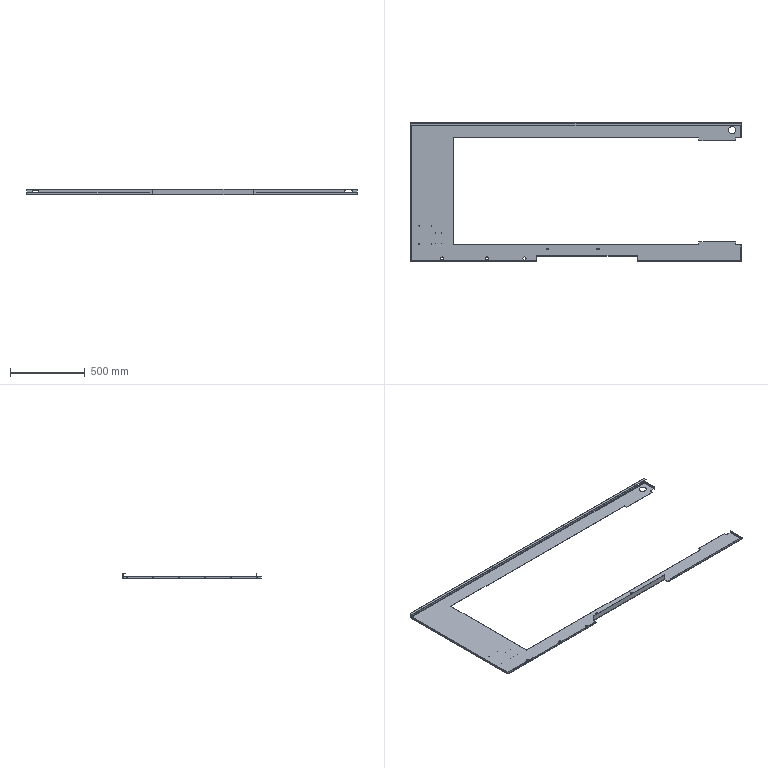Part | NX | features solid 2 | 1 solid | 160 faces | box 2216 x 927.5 x 40 mm | volume 1651301 mm3 | cylinder 82 | plane 78 | commonest cylinder face diameters 1 x16 7 x16 9.2 x14 4 x8 6.2 x8 8 x8